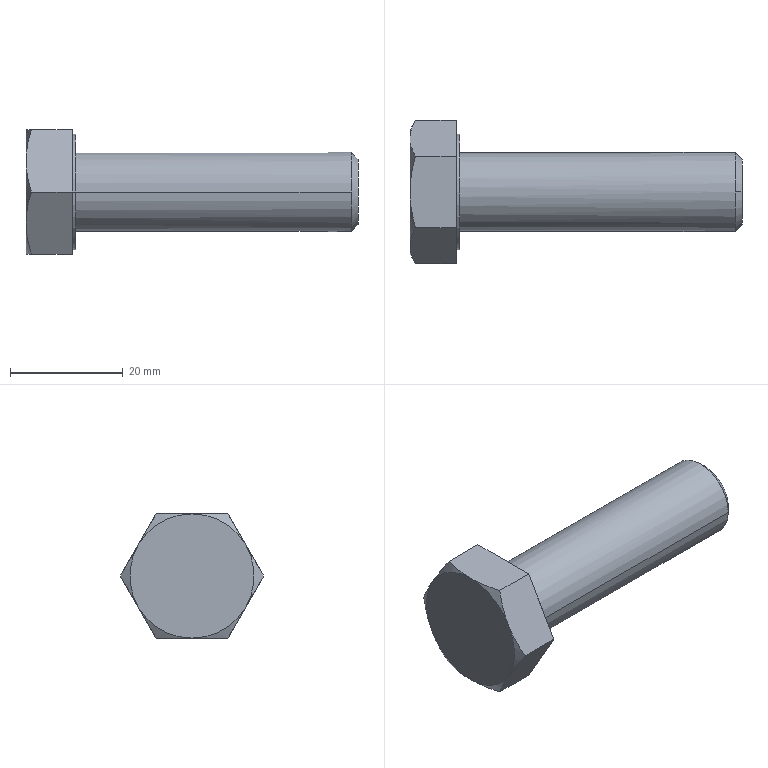Part | STEP file | DIN 931-1 - M14 x 50 | 1 solid | 22 faces | box 58.8 x 25.403 x 22 mm | volume 11289 mm3 | plane 10 | cone 8 | cylinder 4 | commonest cylinder face diameters 14 x2 20.5 x2